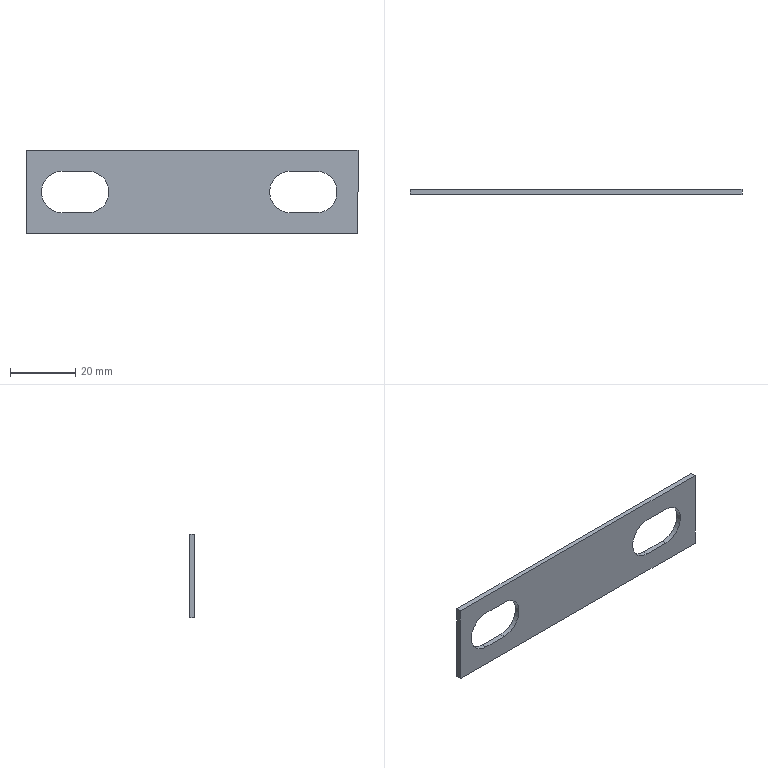Part | SolidWorks | features Extrusion 1 | 1 solid | 14 faces | box 101.6 x 1.524 x 25.4 mm | volume 3238 mm3 | plane 10 | cylinder 4 | commonest cylinder face diameters 12.7 x4
STEP:
#1=CARTESIAN_POINT('',(11.049,1.524,-19.05));
#2=VERTEX_POINT('',#1);
#3=CARTESIAN_POINT('',(11.049,1.524,-6.35));
#4=VERTEX_POINT('',#3);
#5=CARTESIAN_POINT('',(11.049,1.524,-12.7));
#6=DIRECTION('',(0.,1.,0.));
#7=DIRECTION('',(0.,0.,1.));
#8=AXIS2_PLACEMENT_3D('',#5,#6,#7);
#9=CIRCLE('',#8,6.35);
#10=EDGE_CURVE('',#2,#4,#9,.T.);
#11=ORIENTED_EDGE('',*,*,#10,.F.);
#12=CARTESIAN_POINT('',(19.019,1.524,-19.05));
#13=VERTEX_POINT('',#12);
#14=CARTESIAN_POINT('',(11.049,1.524,-19.05));
#15=DIRECTION('',(-1.,0.,0.));
#16=VECTOR('',#15,1000.);
#17=LINE('',#14,#16);
#18=EDGE_CURVE('',#13,#2,#17,.T.);
#19=ORIENTED_EDGE('',*,*,#18,.F.);
#20=CARTESIAN_POINT('',(19.019,1.524,-6.35));
#21=VERTEX_POINT('',#20);
#22=CARTESIAN_POINT('',(19.019,1.524,-12.7));
#23=DIRECTION('',(0.,1.,0.));
#24=DIRECTION('',(0.,0.,1.));
#25=AXIS2_PLACEMENT_3D('',#22,#23,#24);
#26=CIRCLE('',#25,6.35);
#27=EDGE_CURVE('',#21,#13,#26,.T.);
#28=ORIENTED_EDGE('',*,*,#27,.F.);
#29=CARTESIAN_POINT('',(11.049,1.524,-6.35));
#30=DIRECTION('',(1.,0.,0.));
#31=VECTOR('',#30,1000.);
#32=LINE('',#29,#31);
#33=EDGE_CURVE('',#4,#21,#32,.T.);
#34=ORIENTED_EDGE('',*,*,#33,.F.);
#35=EDGE_LOOP('',(#11,#19,#28,#34));
#36=FACE_BOUND('',#35,.T.);
#37=CARTESIAN_POINT('',(0.,1.524,-25.4));
#38=VERTEX_POINT('',#37);
#39=CARTESIAN_POINT('',(0.,1.524,0.));
#40=VERTEX_POINT('',#39);
#41=CARTESIAN_POINT('',(0.,1.524,0.));
#42=DIRECTION('',(0.,0.,1.));
#43=VECTOR('',#42,1000.);
#44=LINE('',#41,#43);
#45=EDGE_CURVE('',#38,#40,#44,.T.);
#46=ORIENTED_EDGE('',*,*,#45,.T.);
#47=CARTESIAN_POINT('',(101.6,1.524,0.));
#48=VERTEX_POINT('',#47);
#49=CARTESIAN_POINT('',(0.,1.524,0.));
#50=DIRECTION('',(1.,0.,0.));
#51=VECTOR('',#50,1000.);
#52=LINE('',#49,#51);
#53=EDGE_CURVE('',#40,#48,#52,.T.);
#54=ORIENTED_EDGE('',*,*,#53,.T.);
#55=CARTESIAN_POINT('',(101.6,1.524,-25.4));
#56=VERTEX_POINT('',#55);
#57=CARTESIAN_POINT('',(101.6,1.524,0.));
#58=DIRECTION('',(0.,0.,-1.));
#59=VECTOR('',#58,1000.);
#60=LINE('',#57,#59);
#61=EDGE_CURVE('',#48,#56,#60,.T.);
#62=ORIENTED_EDGE('',*,*,#61,.T.);
#63=CARTESIAN_POINT('',(0.,1.524,-25.4));
#64=DIRECTION('',(-1.,0.,0.));
#65=VECTOR('',#64,1000.);
#66=LINE('',#63,#65);
#67=EDGE_CURVE('',#56,#38,#66,.T.);
#68=ORIENTED_EDGE('',*,*,#67,.T.);
#69=EDGE_LOOP('',(#46,#54,#62,#68));
#70=FACE_OUTER_BOUND('',#69,.T.);
#71=CARTESIAN_POINT('',(80.899,1.524,-19.05));
#72=VERTEX_POINT('',#71);
#73=CARTESIAN_POINT('',(80.899,1.524,-6.35));
#74=VERTEX_POINT('',#73);
#75=CARTESIAN_POINT('',(80.899,1.524,-12.7));
#76=DIRECTION('',(0.,1.,0.));
#77=DIRECTION('',(0.,0.,1.));
#78=AXIS2_PLACEMENT_3D('',#75,#76,#77);
#79=CIRCLE('',#78,6.35);
#80=EDGE_CURVE('',#72,#74,#79,.T.);
#81=ORIENTED_EDGE('',*,*,#80,.F.);
#82=CARTESIAN_POINT('',(88.869,1.524,-19.05));
#83=VERTEX_POINT('',#82);
#84=CARTESIAN_POINT('',(80.899,1.524,-19.05));
#85=DIRECTION('',(-1.,0.,0.));
#86=VECTOR('',#85,1000.);
#87=LINE('',#84,#86);
#88=EDGE_CURVE('',#83,#72,#87,.T.);
#89=ORIENTED_EDGE('',*,*,#88,.F.);
#90=CARTESIAN_POINT('',(88.869,1.524,-6.35));
#91=VERTEX_POINT('',#90);
#92=CARTESIAN_POINT('',(88.869,1.524,-12.7));
#93=DIRECTION('',(0.,1.,0.));
#94=DIRECTION('',(0.,0.,1.));
#95=AXIS2_PLACEMENT_3D('',#92,#93,#94);
#96=CIRCLE('',#95,6.35);
#97=EDGE_CURVE('',#91,#83,#96,.T.);
#98=ORIENTED_EDGE('',*,*,#97,.F.);
#99=CARTESIAN_POINT('',(80.899,1.524,-6.35));
#100=DIRECTION('',(1.,0.,0.));
#101=VECTOR('',#100,1000.);
#102=LINE('',#99,#101);
#103=EDGE_CURVE('',#74,#91,#102,.T.);
#104=ORIENTED_EDGE('',*,*,#103,.F.);
#105=EDGE_LOOP('',(#81,#89,#98,#104));
#106=FACE_BOUND('',#105,.T.);
#107=CARTESIAN_POINT('',(0.,1.524,0.));
#108=DIRECTION('',(0.,-1.,0.));
#109=DIRECTION('',(0.,0.,-1.));
#110=AXIS2_PLACEMENT_3D('',#107,#108,#109);
#111=PLANE('',#110);
#112=ADVANCED_FACE('',(#36,#70,#106),#111,.F.);
#113=CARTESIAN_POINT('',(19.019,0.,-19.05));
#114=VERTEX_POINT('',#113);
#115=CARTESIAN_POINT('',(11.049,0.,-19.05));
#116=VERTEX_POINT('',#115);
#117=CARTESIAN_POINT('',(11.049,0.,-19.05));
#118=DIRECTION('',(-1.,0.,0.));
#119=VECTOR('',#118,1000.);
#120=LINE('',#117,#119);
#121=EDGE_CURVE('',#114,#116,#120,.T.);
#122=ORIENTED_EDGE('',*,*,#121,.T.);
#123=CARTESIAN_POINT('',(11.049,0.,-6.35));
#124=VERTEX_POINT('',#123);
#125=CARTESIAN_POINT('',(11.049,0.,-12.7));
#126=DIRECTION('',(0.,1.,0.));
#127=DIRECTION('',(0.,0.,1.));
#128=AXIS2_PLACEMENT_3D('',#125,#126,#127);
#129=CIRCLE('',#128,6.35);
#130=EDGE_CURVE('',#116,#124,#129,.T.);
#131=ORIENTED_EDGE('',*,*,#130,.T.);
#132=CARTESIAN_POINT('',(19.019,0.,-6.35));
#133=VERTEX_POINT('',#132);
#134=CARTESIAN_POINT('',(11.049,0.,-6.35));
#135=DIRECTION('',(1.,0.,0.));
#136=VECTOR('',#135,1000.);
#137=LINE('',#134,#136);
#138=EDGE_CURVE('',#124,#133,#137,.T.);
#139=ORIENTED_EDGE('',*,*,#138,.T.);
#140=CARTESIAN_POINT('',(19.019,0.,-12.7));
#141=DIRECTION('',(0.,1.,0.));
#142=DIRECTION('',(0.,0.,1.));
#143=AXIS2_PLACEMENT_3D('',#140,#141,#142);
#144=CIRCLE('',#143,6.35);
#145=EDGE_CURVE('',#133,#114,#144,.T.);
#146=ORIENTED_EDGE('',*,*,#145,.T.);
#147=EDGE_LOOP('',(#122,#131,#139,#146));
#148=FACE_BOUND('',#147,.T.);
#149=CARTESIAN_POINT('',(0.,0.,-25.4));
#150=VERTEX_POINT('',#149);
#151=CARTESIAN_POINT('',(0.,0.,0.));
#152=VERTEX_POINT('',#151);
#153=CARTESIAN_POINT('',(0.,0.,0.));
#154=DIRECTION('',(0.,0.,1.));
#155=VECTOR('',#154,1000.);
#156=LINE('',#153,#155);
#157=EDGE_CURVE('',#150,#152,#156,.T.);
#158=ORIENTED_EDGE('',*,*,#157,.F.);
#159=CARTESIAN_POINT('',(101.6,0.,-25.4));
#160=VERTEX_POINT('',#159);
#161=CARTESIAN_POINT('',(0.,0.,-25.4));
#162=DIRECTION('',(-1.,0.,0.));
#163=VECTOR('',#162,1000.);
#164=LINE('',#161,#163);
#165=EDGE_CURVE('',#160,#150,#164,.T.);
#166=ORIENTED_EDGE('',*,*,#165,.F.);
#167=CARTESIAN_POINT('',(101.6,0.,0.));
#168=VERTEX_POINT('',#167);
#169=CARTESIAN_POINT('',(101.6,0.,0.));
#170=DIRECTION('',(0.,0.,-1.));
#171=VECTOR('',#170,1000.);
#172=LINE('',#169,#171);
#173=EDGE_CURVE('',#168,#160,#172,.T.);
#174=ORIENTED_EDGE('',*,*,#173,.F.);
#175=CARTESIAN_POINT('',(0.,0.,0.));
#176=DIRECTION('',(1.,0.,0.));
#177=VECTOR('',#176,1000.);
#178=LINE('',#175,#177);
#179=EDGE_CURVE('',#152,#168,#178,.T.);
#180=ORIENTED_EDGE('',*,*,#179,.F.);
#181=EDGE_LOOP('',(#158,#166,#174,#180));
#182=FACE_OUTER_BOUND('',#181,.T.);
#183=CARTESIAN_POINT('',(88.869,0.,-19.05));
#184=VERTEX_POINT('',#183);
#185=CARTESIAN_POINT('',(80.899,0.,-19.05));
#186=VERTEX_POINT('',#185);
#187=CARTESIAN_POINT('',(80.899,0.,-19.05));
#188=DIRECTION('',(-1.,0.,0.));
#189=VECTOR('',#188,1000.);
#190=LINE('',#187,#189);
#191=EDGE_CURVE('',#184,#186,#190,.T.);
#192=ORIENTED_EDGE('',*,*,#191,.T.);
#193=CARTESIAN_POINT('',(80.899,0.,-6.35));
#194=VERTEX_POINT('',#193);
#195=CARTESIAN_POINT('',(80.899,0.,-12.7));
#196=DIRECTION('',(0.,1.,0.));
#197=DIRECTION('',(0.,0.,1.));
#198=AXIS2_PLACEMENT_3D('',#195,#196,#197);
#199=CIRCLE('',#198,6.35);
#200=EDGE_CURVE('',#186,#194,#199,.T.);
#201=ORIENTED_EDGE('',*,*,#200,.T.);
#202=CARTESIAN_POINT('',(88.869,0.,-6.35));
#203=VERTEX_POINT('',#202);
#204=CARTESIAN_POINT('',(80.899,0.,-6.35));
#205=DIRECTION('',(1.,0.,0.));
#206=VECTOR('',#205,1000.);
#207=LINE('',#204,#206);
#208=EDGE_CURVE('',#194,#203,#207,.T.);
#209=ORIENTED_EDGE('',*,*,#208,.T.);
#210=CARTESIAN_POINT('',(88.869,0.,-12.7));
#211=DIRECTION('',(0.,1.,0.));
#212=DIRECTION('',(0.,0.,1.));
#213=AXIS2_PLACEMENT_3D('',#210,#211,#212);
#214=CIRCLE('',#213,6.35);
#215=EDGE_CURVE('',#203,#184,#214,.T.);
#216=ORIENTED_EDGE('',*,*,#215,.T.);
#217=EDGE_LOOP('',(#192,#201,#209,#216));
#218=FACE_BOUND('',#217,.T.);
#219=CARTESIAN_POINT('',(0.,0.,0.));
#220=DIRECTION('',(0.,-1.,0.));
#221=DIRECTION('',(0.,0.,-1.));
#222=AXIS2_PLACEMENT_3D('',#219,#220,#221);
#223=PLANE('',#222);
#224=ADVANCED_FACE('',(#148,#182,#218),#223,.T.);
#225=ORIENTED_EDGE('',*,*,#157,.T.);
#226=CARTESIAN_POINT('',(0.,1.524,0.));
#227=DIRECTION('',(0.,-1.,0.));
#228=VECTOR('',#227,1000.);
#229=LINE('',#226,#228);
#230=EDGE_CURVE('',#40,#152,#229,.T.);
#231=ORIENTED_EDGE('',*,*,#230,.F.);
#232=ORIENTED_EDGE('',*,*,#45,.F.);
#233=CARTESIAN_POINT('',(0.,1.524,-25.4));
#234=DIRECTION('',(0.,-1.,0.));
#235=VECTOR('',#234,1000.);
#236=LINE('',#233,#235);
#237=EDGE_CURVE('',#38,#150,#236,.T.);
#238=ORIENTED_EDGE('',*,*,#237,.T.);
#239=EDGE_LOOP('',(#225,#231,#232,#238));
#240=FACE_OUTER_BOUND('',#239,.T.);
#241=CARTESIAN_POINT('',(0.,1.524,0.));
#242=DIRECTION('',(1.,0.,0.));
#243=DIRECTION('',(0.,0.,-1.));
#244=AXIS2_PLACEMENT_3D('',#241,#242,#243);
#245=PLANE('',#244);
#246=ADVANCED_FACE('',(#240),#245,.F.);
#247=ORIENTED_EDGE('',*,*,#179,.T.);
#248=CARTESIAN_POINT('',(101.6,1.524,0.));
#249=DIRECTION('',(0.,-1.,0.));
#250=VECTOR('',#249,1000.);
#251=LINE('',#248,#250);
#252=EDGE_CURVE('',#48,#168,#251,.T.);
#253=ORIENTED_EDGE('',*,*,#252,.F.);
#254=ORIENTED_EDGE('',*,*,#53,.F.);
#255=ORIENTED_EDGE('',*,*,#230,.T.);
#256=EDGE_LOOP('',(#247,#253,#254,#255));
#257=FACE_OUTER_BOUND('',#256,.T.);
#258=CARTESIAN_POINT('',(0.,1.524,0.));
#259=DIRECTION('',(0.,0.,-1.));
#260=DIRECTION('',(-1.,0.,0.));
#261=AXIS2_PLACEMENT_3D('',#258,#259,#260);
#262=PLANE('',#261);
#263=ADVANCED_FACE('',(#257),#262,.F.);
#264=ORIENTED_EDGE('',*,*,#173,.T.);
#265=CARTESIAN_POINT('',(101.6,1.524,-25.4));
#266=DIRECTION('',(0.,-1.,0.));
#267=VECTOR('',#266,1000.);
#268=LINE('',#265,#267);
#269=EDGE_CURVE('',#56,#160,#268,.T.);
#270=ORIENTED_EDGE('',*,*,#269,.F.);
#271=ORIENTED_EDGE('',*,*,#61,.F.);
#272=ORIENTED_EDGE('',*,*,#252,.T.);
#273=EDGE_LOOP('',(#264,#270,#271,#272));
#274=FACE_OUTER_BOUND('',#273,.T.);
#275=CARTESIAN_POINT('',(101.6,1.524,0.));
#276=DIRECTION('',(-1.,0.,0.));
#277=DIRECTION('',(0.,0.,1.));
#278=AXIS2_PLACEMENT_3D('',#275,#276,#277);
#279=PLANE('',#278);
#280=ADVANCED_FACE('',(#274),#279,.F.);
#281=ORIENTED_EDGE('',*,*,#165,.T.);
#282=ORIENTED_EDGE('',*,*,#237,.F.);
#283=ORIENTED_EDGE('',*,*,#67,.F.);
#284=ORIENTED_EDGE('',*,*,#269,.T.);
#285=EDGE_LOOP('',(#281,#282,#283,#284));
#286=FACE_OUTER_BOUND('',#285,.T.);
#287=CARTESIAN_POINT('',(0.,1.524,-25.4));
#288=DIRECTION('',(0.,0.,1.));
#289=DIRECTION('',(1.,0.,0.));
#290=AXIS2_PLACEMENT_3D('',#287,#288,#289);
#291=PLANE('',#290);
#292=ADVANCED_FACE('',(#286),#291,.F.);
#293=ORIENTED_EDGE('',*,*,#130,.F.);
#294=CARTESIAN_POINT('',(11.049,1.524,-19.05));
#295=DIRECTION('',(0.,-1.,0.));
#296=VECTOR('',#295,1000.);
#297=LINE('',#294,#296);
#298=EDGE_CURVE('',#2,#116,#297,.T.);
#299=ORIENTED_EDGE('',*,*,#298,.F.);
#300=ORIENTED_EDGE('',*,*,#10,.T.);
#301=CARTESIAN_POINT('',(11.049,1.524,-6.35));
#302=DIRECTION('',(0.,-1.,0.));
#303=VECTOR('',#302,1000.);
#304=LINE('',#301,#303);
#305=EDGE_CURVE('',#4,#124,#304,.T.);
#306=ORIENTED_EDGE('',*,*,#305,.T.);
#307=EDGE_LOOP('',(#293,#299,#300,#306));
#308=FACE_OUTER_BOUND('',#307,.T.);
#309=CARTESIAN_POINT('',(11.049,1.524,-12.7));
#310=DIRECTION('',(0.,-1.,0.));
#311=DIRECTION('',(0.,0.,-1.));
#312=AXIS2_PLACEMENT_3D('',#309,#310,#311);
#313=CYLINDRICAL_SURFACE('',#312,6.35);
#314=ADVANCED_FACE('',(#308),#313,.F.);
#315=ORIENTED_EDGE('',*,*,#138,.F.);
#316=ORIENTED_EDGE('',*,*,#305,.F.);
#317=ORIENTED_EDGE('',*,*,#33,.T.);
#318=CARTESIAN_POINT('',(19.019,1.524,-6.35));
#319=DIRECTION('',(0.,-1.,0.));
#320=VECTOR('',#319,1000.);
#321=LINE('',#318,#320);
#322=EDGE_CURVE('',#21,#133,#321,.T.);
#323=ORIENTED_EDGE('',*,*,#322,.T.);
#324=EDGE_LOOP('',(#315,#316,#317,#323));
#325=FACE_OUTER_BOUND('',#324,.T.);
#326=CARTESIAN_POINT('',(11.049,1.524,-6.35));
#327=DIRECTION('',(0.,0.,-1.));
#328=DIRECTION('',(-1.,0.,0.));
#329=AXIS2_PLACEMENT_3D('',#326,#327,#328);
#330=PLANE('',#329);
#331=ADVANCED_FACE('',(#325),#330,.T.);
#332=ORIENTED_EDGE('',*,*,#145,.F.);
#333=ORIENTED_EDGE('',*,*,#322,.F.);
#334=ORIENTED_EDGE('',*,*,#27,.T.);
#335=CARTESIAN_POINT('',(19.019,1.524,-19.05));
#336=DIRECTION('',(0.,-1.,0.));
#337=VECTOR('',#336,1000.);
#338=LINE('',#335,#337);
#339=EDGE_CURVE('',#13,#114,#338,.T.);
#340=ORIENTED_EDGE('',*,*,#339,.T.);
#341=EDGE_LOOP('',(#332,#333,#334,#340));
#342=FACE_OUTER_BOUND('',#341,.T.);
#343=CARTESIAN_POINT('',(19.019,1.524,-12.7));
#344=DIRECTION('',(0.,-1.,0.));
#345=DIRECTION('',(0.,0.,-1.));
#346=AXIS2_PLACEMENT_3D('',#343,#344,#345);
#347=CYLINDRICAL_SURFACE('',#346,6.35);
#348=ADVANCED_FACE('',(#342),#347,.F.);
#349=ORIENTED_EDGE('',*,*,#121,.F.);
#350=ORIENTED_EDGE('',*,*,#339,.F.);
#351=ORIENTED_EDGE('',*,*,#18,.T.);
#352=ORIENTED_EDGE('',*,*,#298,.T.);
#353=EDGE_LOOP('',(#349,#350,#351,#352));
#354=FACE_OUTER_BOUND('',#353,.T.);
#355=CARTESIAN_POINT('',(11.049,1.524,-19.05));
#356=DIRECTION('',(0.,0.,1.));
#357=DIRECTION('',(1.,0.,0.));
#358=AXIS2_PLACEMENT_3D('',#355,#356,#357);
#359=PLANE('',#358);
#360=ADVANCED_FACE('',(#354),#359,.T.);
#361=ORIENTED_EDGE('',*,*,#200,.F.);
#362=CARTESIAN_POINT('',(80.899,1.524,-19.05));
#363=DIRECTION('',(0.,-1.,0.));
#364=VECTOR('',#363,1000.);
#365=LINE('',#362,#364);
#366=EDGE_CURVE('',#72,#186,#365,.T.);
#367=ORIENTED_EDGE('',*,*,#366,.F.);
#368=ORIENTED_EDGE('',*,*,#80,.T.);
#369=CARTESIAN_POINT('',(80.899,1.524,-6.35));
#370=DIRECTION('',(0.,-1.,0.));
#371=VECTOR('',#370,1000.);
#372=LINE('',#369,#371);
#373=EDGE_CURVE('',#74,#194,#372,.T.);
#374=ORIENTED_EDGE('',*,*,#373,.T.);
#375=EDGE_LOOP('',(#361,#367,#368,#374));
#376=FACE_OUTER_BOUND('',#375,.T.);
#377=CARTESIAN_POINT('',(80.899,1.524,-12.7));
#378=DIRECTION('',(0.,-1.,0.));
#379=DIRECTION('',(0.,0.,-1.));
#380=AXIS2_PLACEMENT_3D('',#377,#378,#379);
#381=CYLINDRICAL_SURFACE('',#380,6.35);
#382=ADVANCED_FACE('',(#376),#381,.F.);
#383=ORIENTED_EDGE('',*,*,#208,.F.);
#384=ORIENTED_EDGE('',*,*,#373,.F.);
#385=ORIENTED_EDGE('',*,*,#103,.T.);
#386=CARTESIAN_POINT('',(88.869,1.524,-6.35));
#387=DIRECTION('',(0.,-1.,0.));
#388=VECTOR('',#387,1000.);
#389=LINE('',#386,#388);
#390=EDGE_CURVE('',#91,#203,#389,.T.);
#391=ORIENTED_EDGE('',*,*,#390,.T.);
#392=EDGE_LOOP('',(#383,#384,#385,#391));
#393=FACE_OUTER_BOUND('',#392,.T.);
#394=CARTESIAN_POINT('',(80.899,1.524,-6.35));
#395=DIRECTION('',(0.,0.,-1.));
#396=DIRECTION('',(-1.,0.,0.));
#397=AXIS2_PLACEMENT_3D('',#394,#395,#396);
#398=PLANE('',#397);
#399=ADVANCED_FACE('',(#393),#398,.T.);
#400=ORIENTED_EDGE('',*,*,#215,.F.);
#401=ORIENTED_EDGE('',*,*,#390,.F.);
#402=ORIENTED_EDGE('',*,*,#97,.T.);
#403=CARTESIAN_POINT('',(88.869,1.524,-19.05));
#404=DIRECTION('',(0.,-1.,0.));
#405=VECTOR('',#404,1000.);
#406=LINE('',#403,#405);
#407=EDGE_CURVE('',#83,#184,#406,.T.);
#408=ORIENTED_EDGE('',*,*,#407,.T.);
#409=EDGE_LOOP('',(#400,#401,#402,#408));
#410=FACE_OUTER_BOUND('',#409,.T.);
#411=CARTESIAN_POINT('',(88.869,1.524,-12.7));
#412=DIRECTION('',(0.,-1.,0.));
#413=DIRECTION('',(0.,0.,-1.));
#414=AXIS2_PLACEMENT_3D('',#411,#412,#413);
#415=CYLINDRICAL_SURFACE('',#414,6.35);
#416=ADVANCED_FACE('',(#410),#415,.F.);
#417=ORIENTED_EDGE('',*,*,#191,.F.);
#418=ORIENTED_EDGE('',*,*,#407,.F.);
#419=ORIENTED_EDGE('',*,*,#88,.T.);
#420=ORIENTED_EDGE('',*,*,#366,.T.);
#421=EDGE_LOOP('',(#417,#418,#419,#420));
#422=FACE_OUTER_BOUND('',#421,.T.);
#423=CARTESIAN_POINT('',(80.899,1.524,-19.05));
#424=DIRECTION('',(0.,0.,1.));
#425=DIRECTION('',(1.,0.,0.));
#426=AXIS2_PLACEMENT_3D('',#423,#424,#425);
#427=PLANE('',#426);
#428=ADVANCED_FACE('',(#422),#427,.T.);
#429=CLOSED_SHELL('',(#112,#224,#246,#263,#280,#292,#314,#331,#348,#360,#382,#399,#416,#428));
#430=MANIFOLD_SOLID_BREP('',#429);
#431=CARTESIAN_POINT('',(0.,0.,0.));
#432=DIRECTION('',(0.,0.,1.));
#433=DIRECTION('',(1.,0.,0.));
#434=AXIS2_PLACEMENT_3D('',#431,#432,#433);
#435=(LENGTH_UNIT()NAMED_UNIT(*)SI_UNIT(.MILLI.,.METRE.));
#436=UNCERTAINTY_MEASURE_WITH_UNIT(LENGTH_MEASURE(0.00001),#435,'','');
#437=(NAMED_UNIT(*)PLANE_ANGLE_UNIT()SI_UNIT($,.RADIAN.));
#438=(NAMED_UNIT(*)SI_UNIT($,.STERADIAN.)SOLID_ANGLE_UNIT());
#439=(GEOMETRIC_REPRESENTATION_CONTEXT(3)GLOBAL_UNCERTAINTY_ASSIGNED_CONTEXT((#436))GLOBAL_UNIT_ASSIGNED_CONTEXT((#435,#437,#438))REPRESENTATION_CONTEXT('',''));
#440=ADVANCED_BREP_SHAPE_REPRESENTATION('',(#430,#434),#439);